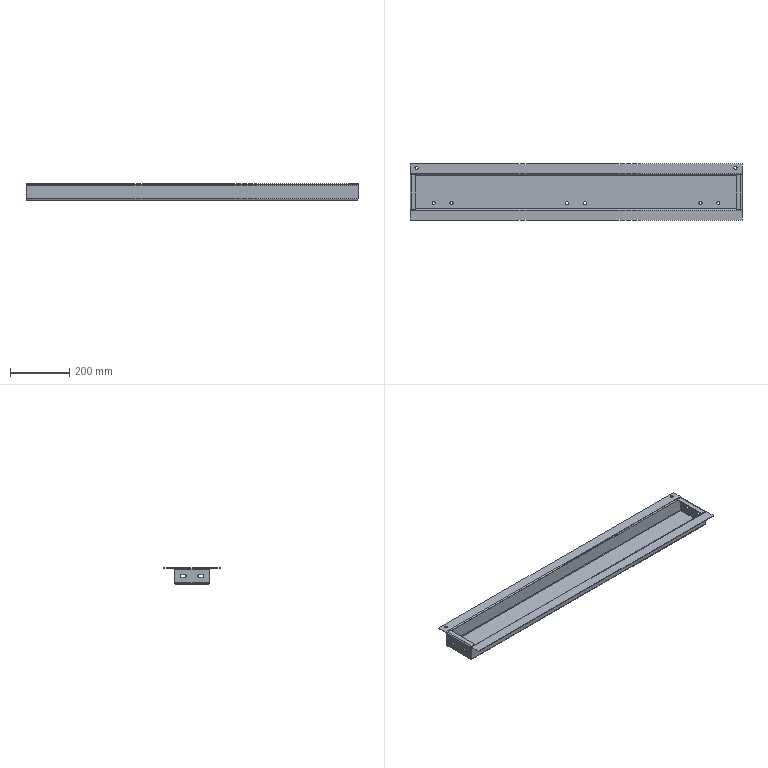Part | STEP file | SYL_0392D6J1SYL0380DJ10-1158695 | 1 solid | 102 faces | box 1120 x 190 x 55 mm | volume 680109 mm3 | plane 54 | cylinder 40 | spline 8 | commonest cylinder face diameters 10.5 x16 4 x8 8 x8 10 x8